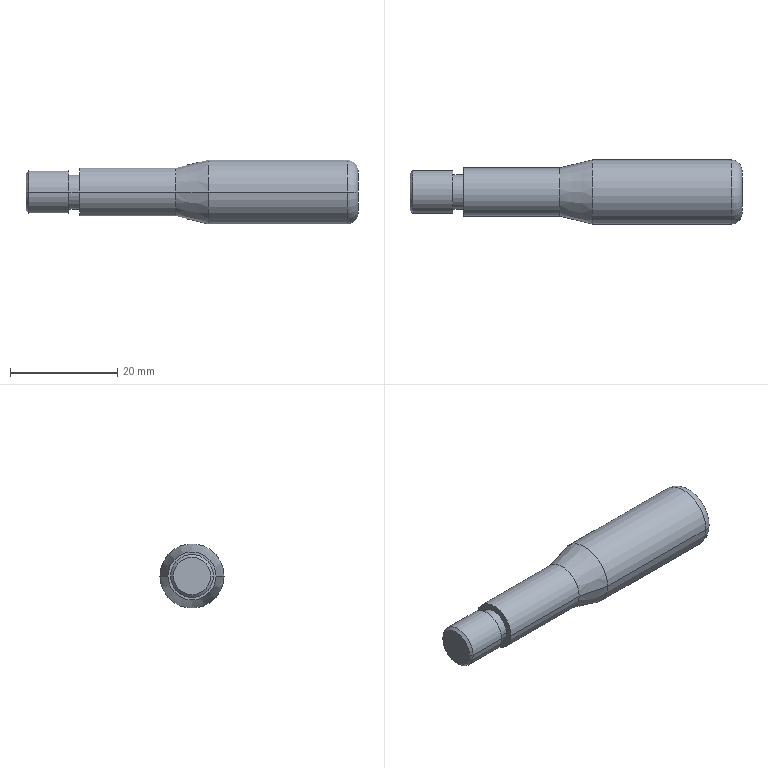Part | SolidWorks | features Chamfer 1, Fillet 1, Revolution 1 | 1 solid | 18 faces | box 62 x 12 x 12 mm | volume 5270 mm3 | cylinder 8 | cone 4 | plane 4 | torus 2 | commonest cylinder face diameters 6.5 x2 8 x2 9 x2 12 x2
STEP:
#1=CARTESIAN_POINT('',(0.,-3.5,0.));
#2=VERTEX_POINT('',#1);
#3=CARTESIAN_POINT('',(0.,3.5,0.));
#4=VERTEX_POINT('',#3);
#5=CARTESIAN_POINT('',(0.,0.,0.));
#6=DIRECTION('',(-1.,0.,0.));
#7=DIRECTION('',(0.,-1.,0.));
#8=AXIS2_PLACEMENT_3D('',#5,#6,#7);
#9=CIRCLE('',#8,3.5);
#10=EDGE_CURVE('',#2,#4,#9,.T.);
#11=ORIENTED_EDGE('',*,*,#10,.F.);
#12=CARTESIAN_POINT('',(0.5,-4.,0.));
#13=VERTEX_POINT('',#12);
#14=CARTESIAN_POINT('',(0.5,-4.,0.));
#15=DIRECTION('',(0.7071,-0.7071,0.));
#16=VECTOR('',#15,1000.);
#17=LINE('',#14,#16);
#18=EDGE_CURVE('',#2,#13,#17,.T.);
#19=ORIENTED_EDGE('',*,*,#18,.T.);
#20=CARTESIAN_POINT('',(0.5,4.,0.));
#21=VERTEX_POINT('',#20);
#22=CARTESIAN_POINT('',(0.5,0.,0.));
#23=DIRECTION('',(1.,0.,0.));
#24=DIRECTION('',(0.,-1.,0.));
#25=AXIS2_PLACEMENT_3D('',#22,#23,#24);
#26=CIRCLE('',#25,4.);
#27=EDGE_CURVE('',#21,#13,#26,.T.);
#28=ORIENTED_EDGE('',*,*,#27,.F.);
#29=CARTESIAN_POINT('',(0.5,4.,0.));
#30=DIRECTION('',(0.7071,0.7071,0.));
#31=VECTOR('',#30,1000.);
#32=LINE('',#29,#31);
#33=EDGE_CURVE('',#4,#21,#32,.T.);
#34=ORIENTED_EDGE('',*,*,#33,.F.);
#35=EDGE_LOOP('',(#11,#19,#28,#34));
#36=FACE_OUTER_BOUND('',#35,.T.);
#37=CARTESIAN_POINT('',(0.5,0.,0.));
#38=DIRECTION('',(1.,0.,0.));
#39=DIRECTION('',(0.,1.,0.));
#40=AXIS2_PLACEMENT_3D('',#37,#38,#39);
#41=CONICAL_SURFACE('',#40,4.,0.7854);
#42=ADVANCED_FACE('',(#36),#41,.T.);
#43=CARTESIAN_POINT('',(60.,-6.,0.));
#44=VERTEX_POINT('',#43);
#45=CARTESIAN_POINT('',(60.,6.,0.));
#46=VERTEX_POINT('',#45);
#47=CARTESIAN_POINT('',(60.,0.,0.));
#48=DIRECTION('',(-1.,0.,0.));
#49=DIRECTION('',(0.,1.,0.));
#50=AXIS2_PLACEMENT_3D('',#47,#48,#49);
#51=CIRCLE('',#50,6.);
#52=EDGE_CURVE('',#44,#46,#51,.T.);
#53=ORIENTED_EDGE('',*,*,#52,.F.);
#54=CARTESIAN_POINT('',(62.,-4.,0.));
#55=VERTEX_POINT('',#54);
#56=CARTESIAN_POINT('',(60.,-4.,0.));
#57=DIRECTION('',(0.,0.,1.));
#58=DIRECTION('',(0.,-1.,0.));
#59=AXIS2_PLACEMENT_3D('',#56,#57,#58);
#60=CIRCLE('',#59,2.);
#61=EDGE_CURVE('',#44,#55,#60,.T.);
#62=ORIENTED_EDGE('',*,*,#61,.T.);
#63=CARTESIAN_POINT('',(62.,4.,0.));
#64=VERTEX_POINT('',#63);
#65=CARTESIAN_POINT('',(62.,0.,0.));
#66=DIRECTION('',(1.,0.,0.));
#67=DIRECTION('',(0.,1.,0.));
#68=AXIS2_PLACEMENT_3D('',#65,#66,#67);
#69=CIRCLE('',#68,4.);
#70=EDGE_CURVE('',#64,#55,#69,.T.);
#71=ORIENTED_EDGE('',*,*,#70,.F.);
#72=CARTESIAN_POINT('',(60.,4.,0.));
#73=DIRECTION('',(0.,0.,-1.));
#74=DIRECTION('',(-1.,0.,0.));
#75=AXIS2_PLACEMENT_3D('',#72,#73,#74);
#76=CIRCLE('',#75,2.);
#77=EDGE_CURVE('',#46,#64,#76,.T.);
#78=ORIENTED_EDGE('',*,*,#77,.F.);
#79=EDGE_LOOP('',(#53,#62,#71,#78));
#80=FACE_OUTER_BOUND('',#79,.T.);
#81=CARTESIAN_POINT('',(60.,0.,0.));
#82=DIRECTION('',(1.,0.,0.));
#83=DIRECTION('',(0.,1.,0.));
#84=AXIS2_PLACEMENT_3D('',#81,#82,#83);
#85=TOROIDAL_SURFACE('',#84,4.,2.);
#86=ADVANCED_FACE('',(#80),#85,.T.);
#87=CARTESIAN_POINT('',(34.,6.,0.));
#88=VERTEX_POINT('',#87);
#89=CARTESIAN_POINT('',(34.,-6.,0.));
#90=VERTEX_POINT('',#89);
#91=CARTESIAN_POINT('',(34.,0.,0.));
#92=DIRECTION('',(1.,0.,0.));
#93=DIRECTION('',(0.,1.,0.));
#94=AXIS2_PLACEMENT_3D('',#91,#92,#93);
#95=CIRCLE('',#94,6.);
#96=EDGE_CURVE('',#88,#90,#95,.T.);
#97=ORIENTED_EDGE('',*,*,#96,.T.);
#98=CARTESIAN_POINT('',(62.,-6.,0.));
#99=DIRECTION('',(1.,0.,0.));
#100=VECTOR('',#99,1000.);
#101=LINE('',#98,#100);
#102=EDGE_CURVE('',#90,#44,#101,.T.);
#103=ORIENTED_EDGE('',*,*,#102,.T.);
#104=ORIENTED_EDGE('',*,*,#52,.T.);
#105=CARTESIAN_POINT('',(62.,6.,0.));
#106=DIRECTION('',(1.,0.,0.));
#107=VECTOR('',#106,1000.);
#108=LINE('',#105,#107);
#109=EDGE_CURVE('',#88,#46,#108,.T.);
#110=ORIENTED_EDGE('',*,*,#109,.F.);
#111=EDGE_LOOP('',(#97,#103,#104,#110));
#112=FACE_OUTER_BOUND('',#111,.T.);
#113=CARTESIAN_POINT('',(62.,0.,0.));
#114=DIRECTION('',(1.,0.,0.));
#115=DIRECTION('',(0.,1.,0.));
#116=AXIS2_PLACEMENT_3D('',#113,#114,#115);
#117=CYLINDRICAL_SURFACE('',#116,6.);
#118=ADVANCED_FACE('',(#112),#117,.T.);
#119=CARTESIAN_POINT('',(28.,4.5,0.));
#120=VERTEX_POINT('',#119);
#121=CARTESIAN_POINT('',(28.,-4.5,0.));
#122=VERTEX_POINT('',#121);
#123=CARTESIAN_POINT('',(28.,0.,0.));
#124=DIRECTION('',(1.,0.,0.));
#125=DIRECTION('',(0.,1.,0.));
#126=AXIS2_PLACEMENT_3D('',#123,#124,#125);
#127=CIRCLE('',#126,4.5);
#128=EDGE_CURVE('',#120,#122,#127,.T.);
#129=ORIENTED_EDGE('',*,*,#128,.T.);
#130=CARTESIAN_POINT('',(34.,-6.,0.));
#131=DIRECTION('',(0.9701,-0.2425,0.));
#132=VECTOR('',#131,1000.);
#133=LINE('',#130,#132);
#134=EDGE_CURVE('',#122,#90,#133,.T.);
#135=ORIENTED_EDGE('',*,*,#134,.T.);
#136=ORIENTED_EDGE('',*,*,#96,.F.);
#137=CARTESIAN_POINT('',(34.,6.,0.));
#138=DIRECTION('',(0.9701,0.2425,0.));
#139=VECTOR('',#138,1000.);
#140=LINE('',#137,#139);
#141=EDGE_CURVE('',#120,#88,#140,.T.);
#142=ORIENTED_EDGE('',*,*,#141,.F.);
#143=EDGE_LOOP('',(#129,#135,#136,#142));
#144=FACE_OUTER_BOUND('',#143,.T.);
#145=CARTESIAN_POINT('',(34.,0.,0.));
#146=DIRECTION('',(1.,0.,0.));
#147=DIRECTION('',(0.,1.,0.));
#148=AXIS2_PLACEMENT_3D('',#145,#146,#147);
#149=CONICAL_SURFACE('',#148,6.,0.245);
#150=ADVANCED_FACE('',(#144),#149,.T.);
#151=CARTESIAN_POINT('',(10.,4.5,0.));
#152=VERTEX_POINT('',#151);
#153=CARTESIAN_POINT('',(10.,-4.5,0.));
#154=VERTEX_POINT('',#153);
#155=CARTESIAN_POINT('',(10.,0.,0.));
#156=DIRECTION('',(1.,0.,0.));
#157=DIRECTION('',(0.,1.,0.));
#158=AXIS2_PLACEMENT_3D('',#155,#156,#157);
#159=CIRCLE('',#158,4.5);
#160=EDGE_CURVE('',#152,#154,#159,.T.);
#161=ORIENTED_EDGE('',*,*,#160,.T.);
#162=CARTESIAN_POINT('',(62.,-4.5,0.));
#163=DIRECTION('',(1.,0.,0.));
#164=VECTOR('',#163,1000.);
#165=LINE('',#162,#164);
#166=EDGE_CURVE('',#154,#122,#165,.T.);
#167=ORIENTED_EDGE('',*,*,#166,.T.);
#168=ORIENTED_EDGE('',*,*,#128,.F.);
#169=CARTESIAN_POINT('',(62.,4.5,0.));
#170=DIRECTION('',(1.,0.,0.));
#171=VECTOR('',#170,1000.);
#172=LINE('',#169,#171);
#173=EDGE_CURVE('',#152,#120,#172,.T.);
#174=ORIENTED_EDGE('',*,*,#173,.F.);
#175=EDGE_LOOP('',(#161,#167,#168,#174));
#176=FACE_OUTER_BOUND('',#175,.T.);
#177=CARTESIAN_POINT('',(62.,0.,0.));
#178=DIRECTION('',(1.,0.,0.));
#179=DIRECTION('',(0.,1.,0.));
#180=AXIS2_PLACEMENT_3D('',#177,#178,#179);
#181=CYLINDRICAL_SURFACE('',#180,4.5);
#182=ADVANCED_FACE('',(#176),#181,.T.);
#183=CARTESIAN_POINT('',(8.,3.25,0.));
#184=VERTEX_POINT('',#183);
#185=CARTESIAN_POINT('',(8.,-3.25,0.));
#186=VERTEX_POINT('',#185);
#187=CARTESIAN_POINT('',(8.,0.,0.));
#188=DIRECTION('',(1.,0.,0.));
#189=DIRECTION('',(0.,1.,0.));
#190=AXIS2_PLACEMENT_3D('',#187,#188,#189);
#191=CIRCLE('',#190,3.25);
#192=EDGE_CURVE('',#184,#186,#191,.T.);
#193=ORIENTED_EDGE('',*,*,#192,.T.);
#194=CARTESIAN_POINT('',(10.,-3.25,0.));
#195=VERTEX_POINT('',#194);
#196=CARTESIAN_POINT('',(62.,-3.25,0.));
#197=DIRECTION('',(1.,0.,0.));
#198=VECTOR('',#197,1000.);
#199=LINE('',#196,#198);
#200=EDGE_CURVE('',#186,#195,#199,.T.);
#201=ORIENTED_EDGE('',*,*,#200,.T.);
#202=CARTESIAN_POINT('',(10.,3.25,0.));
#203=VERTEX_POINT('',#202);
#204=CARTESIAN_POINT('',(10.,0.,0.));
#205=DIRECTION('',(1.,0.,0.));
#206=DIRECTION('',(0.,1.,0.));
#207=AXIS2_PLACEMENT_3D('',#204,#205,#206);
#208=CIRCLE('',#207,3.25);
#209=EDGE_CURVE('',#203,#195,#208,.T.);
#210=ORIENTED_EDGE('',*,*,#209,.F.);
#211=CARTESIAN_POINT('',(62.,3.25,0.));
#212=DIRECTION('',(1.,0.,0.));
#213=VECTOR('',#212,1000.);
#214=LINE('',#211,#213);
#215=EDGE_CURVE('',#184,#203,#214,.T.);
#216=ORIENTED_EDGE('',*,*,#215,.F.);
#217=EDGE_LOOP('',(#193,#201,#210,#216));
#218=FACE_OUTER_BOUND('',#217,.T.);
#219=CARTESIAN_POINT('',(62.,0.,0.));
#220=DIRECTION('',(1.,0.,0.));
#221=DIRECTION('',(0.,1.,0.));
#222=AXIS2_PLACEMENT_3D('',#219,#220,#221);
#223=CYLINDRICAL_SURFACE('',#222,3.25);
#224=ADVANCED_FACE('',(#218),#223,.T.);
#225=ORIENTED_EDGE('',*,*,#27,.T.);
#226=CARTESIAN_POINT('',(8.,-4.,0.));
#227=VERTEX_POINT('',#226);
#228=CARTESIAN_POINT('',(62.,-4.,0.));
#229=DIRECTION('',(1.,0.,0.));
#230=VECTOR('',#229,1000.);
#231=LINE('',#228,#230);
#232=EDGE_CURVE('',#13,#227,#231,.T.);
#233=ORIENTED_EDGE('',*,*,#232,.T.);
#234=CARTESIAN_POINT('',(8.,4.,0.));
#235=VERTEX_POINT('',#234);
#236=CARTESIAN_POINT('',(8.,0.,0.));
#237=DIRECTION('',(1.,0.,0.));
#238=DIRECTION('',(0.,1.,0.));
#239=AXIS2_PLACEMENT_3D('',#236,#237,#238);
#240=CIRCLE('',#239,4.);
#241=EDGE_CURVE('',#235,#227,#240,.T.);
#242=ORIENTED_EDGE('',*,*,#241,.F.);
#243=CARTESIAN_POINT('',(62.,4.,0.));
#244=DIRECTION('',(1.,0.,0.));
#245=VECTOR('',#244,1000.);
#246=LINE('',#243,#245);
#247=EDGE_CURVE('',#21,#235,#246,.T.);
#248=ORIENTED_EDGE('',*,*,#247,.F.);
#249=EDGE_LOOP('',(#225,#233,#242,#248));
#250=FACE_OUTER_BOUND('',#249,.T.);
#251=CARTESIAN_POINT('',(62.,0.,0.));
#252=DIRECTION('',(1.,0.,0.));
#253=DIRECTION('',(0.,1.,0.));
#254=AXIS2_PLACEMENT_3D('',#251,#252,#253);
#255=CYLINDRICAL_SURFACE('',#254,4.);
#256=ADVANCED_FACE('',(#250),#255,.T.);
#257=CARTESIAN_POINT('',(0.,0.,0.));
#258=DIRECTION('',(-1.,0.,0.));
#259=DIRECTION('',(0.,-1.,0.));
#260=AXIS2_PLACEMENT_3D('',#257,#258,#259);
#261=CIRCLE('',#260,3.5);
#262=EDGE_CURVE('',#4,#2,#261,.T.);
#263=ORIENTED_EDGE('',*,*,#262,.T.);
#264=ORIENTED_EDGE('',*,*,#10,.T.);
#265=EDGE_LOOP('',(#263,#264));
#266=FACE_OUTER_BOUND('',#265,.T.);
#267=CARTESIAN_POINT('',(0.,0.,0.));
#268=DIRECTION('',(-1.,0.,0.));
#269=DIRECTION('',(0.,-1.,0.));
#270=AXIS2_PLACEMENT_3D('',#267,#268,#269);
#271=PLANE('',#270);
#272=ADVANCED_FACE('',(#266),#271,.T.);
#273=ORIENTED_EDGE('',*,*,#232,.F.);
#274=CARTESIAN_POINT('',(0.5,0.,0.));
#275=DIRECTION('',(1.,0.,0.));
#276=DIRECTION('',(0.,-1.,0.));
#277=AXIS2_PLACEMENT_3D('',#274,#275,#276);
#278=CIRCLE('',#277,4.);
#279=EDGE_CURVE('',#13,#21,#278,.T.);
#280=ORIENTED_EDGE('',*,*,#279,.T.);
#281=ORIENTED_EDGE('',*,*,#247,.T.);
#282=CARTESIAN_POINT('',(8.,0.,0.));
#283=DIRECTION('',(1.,0.,0.));
#284=DIRECTION('',(0.,1.,0.));
#285=AXIS2_PLACEMENT_3D('',#282,#283,#284);
#286=CIRCLE('',#285,4.);
#287=EDGE_CURVE('',#227,#235,#286,.T.);
#288=ORIENTED_EDGE('',*,*,#287,.F.);
#289=EDGE_LOOP('',(#273,#280,#281,#288));
#290=FACE_OUTER_BOUND('',#289,.T.);
#291=CARTESIAN_POINT('',(62.,0.,0.));
#292=DIRECTION('',(1.,0.,0.));
#293=DIRECTION('',(0.,1.,0.));
#294=AXIS2_PLACEMENT_3D('',#291,#292,#293);
#295=CYLINDRICAL_SURFACE('',#294,4.);
#296=ADVANCED_FACE('',(#290),#295,.T.);
#297=ORIENTED_EDGE('',*,*,#241,.T.);
#298=ORIENTED_EDGE('',*,*,#287,.T.);
#299=EDGE_LOOP('',(#297,#298));
#300=FACE_OUTER_BOUND('',#299,.T.);
#301=ORIENTED_EDGE('',*,*,#192,.F.);
#302=CARTESIAN_POINT('',(8.,0.,0.));
#303=DIRECTION('',(1.,0.,0.));
#304=DIRECTION('',(0.,1.,0.));
#305=AXIS2_PLACEMENT_3D('',#302,#303,#304);
#306=CIRCLE('',#305,3.25);
#307=EDGE_CURVE('',#186,#184,#306,.T.);
#308=ORIENTED_EDGE('',*,*,#307,.F.);
#309=EDGE_LOOP('',(#301,#308));
#310=FACE_BOUND('',#309,.T.);
#311=CARTESIAN_POINT('',(8.,4.,0.));
#312=DIRECTION('',(1.,0.,0.));
#313=DIRECTION('',(0.,1.,0.));
#314=AXIS2_PLACEMENT_3D('',#311,#312,#313);
#315=PLANE('',#314);
#316=ADVANCED_FACE('',(#300,#310),#315,.T.);
#317=ORIENTED_EDGE('',*,*,#200,.F.);
#318=ORIENTED_EDGE('',*,*,#307,.T.);
#319=ORIENTED_EDGE('',*,*,#215,.T.);
#320=CARTESIAN_POINT('',(10.,0.,0.));
#321=DIRECTION('',(1.,0.,0.));
#322=DIRECTION('',(0.,1.,0.));
#323=AXIS2_PLACEMENT_3D('',#320,#321,#322);
#324=CIRCLE('',#323,3.25);
#325=EDGE_CURVE('',#195,#203,#324,.T.);
#326=ORIENTED_EDGE('',*,*,#325,.F.);
#327=EDGE_LOOP('',(#317,#318,#319,#326));
#328=FACE_OUTER_BOUND('',#327,.T.);
#329=CARTESIAN_POINT('',(62.,0.,0.));
#330=DIRECTION('',(1.,0.,0.));
#331=DIRECTION('',(0.,1.,0.));
#332=AXIS2_PLACEMENT_3D('',#329,#330,#331);
#333=CYLINDRICAL_SURFACE('',#332,3.25);
#334=ADVANCED_FACE('',(#328),#333,.T.);
#335=ORIENTED_EDGE('',*,*,#209,.T.);
#336=ORIENTED_EDGE('',*,*,#325,.T.);
#337=EDGE_LOOP('',(#335,#336));
#338=FACE_BOUND('',#337,.T.);
#339=ORIENTED_EDGE('',*,*,#160,.F.);
#340=CARTESIAN_POINT('',(10.,0.,0.));
#341=DIRECTION('',(1.,0.,0.));
#342=DIRECTION('',(0.,1.,0.));
#343=AXIS2_PLACEMENT_3D('',#340,#341,#342);
#344=CIRCLE('',#343,4.5);
#345=EDGE_CURVE('',#154,#152,#344,.T.);
#346=ORIENTED_EDGE('',*,*,#345,.F.);
#347=EDGE_LOOP('',(#339,#346));
#348=FACE_OUTER_BOUND('',#347,.T.);
#349=CARTESIAN_POINT('',(10.,3.25,0.));
#350=DIRECTION('',(-1.,0.,0.));
#351=DIRECTION('',(0.,-1.,0.));
#352=AXIS2_PLACEMENT_3D('',#349,#350,#351);
#353=PLANE('',#352);
#354=ADVANCED_FACE('',(#338,#348),#353,.T.);
#355=ORIENTED_EDGE('',*,*,#166,.F.);
#356=ORIENTED_EDGE('',*,*,#345,.T.);
#357=ORIENTED_EDGE('',*,*,#173,.T.);
#358=CARTESIAN_POINT('',(28.,0.,0.));
#359=DIRECTION('',(1.,0.,0.));
#360=DIRECTION('',(0.,1.,0.));
#361=AXIS2_PLACEMENT_3D('',#358,#359,#360);
#362=CIRCLE('',#361,4.5);
#363=EDGE_CURVE('',#122,#120,#362,.T.);
#364=ORIENTED_EDGE('',*,*,#363,.F.);
#365=EDGE_LOOP('',(#355,#356,#357,#364));
#366=FACE_OUTER_BOUND('',#365,.T.);
#367=CARTESIAN_POINT('',(62.,0.,0.));
#368=DIRECTION('',(1.,0.,0.));
#369=DIRECTION('',(0.,1.,0.));
#370=AXIS2_PLACEMENT_3D('',#367,#368,#369);
#371=CYLINDRICAL_SURFACE('',#370,4.5);
#372=ADVANCED_FACE('',(#366),#371,.T.);
#373=ORIENTED_EDGE('',*,*,#134,.F.);
#374=ORIENTED_EDGE('',*,*,#363,.T.);
#375=ORIENTED_EDGE('',*,*,#141,.T.);
#376=CARTESIAN_POINT('',(34.,0.,0.));
#377=DIRECTION('',(1.,0.,0.));
#378=DIRECTION('',(0.,1.,0.));
#379=AXIS2_PLACEMENT_3D('',#376,#377,#378);
#380=CIRCLE('',#379,6.);
#381=EDGE_CURVE('',#90,#88,#380,.T.);
#382=ORIENTED_EDGE('',*,*,#381,.F.);
#383=EDGE_LOOP('',(#373,#374,#375,#382));
#384=FACE_OUTER_BOUND('',#383,.T.);
#385=CARTESIAN_POINT('',(34.,0.,0.));
#386=DIRECTION('',(1.,0.,0.));
#387=DIRECTION('',(0.,1.,0.));
#388=AXIS2_PLACEMENT_3D('',#385,#386,#387);
#389=CONICAL_SURFACE('',#388,6.,0.245);
#390=ADVANCED_FACE('',(#384),#389,.T.);
#391=ORIENTED_EDGE('',*,*,#102,.F.);
#392=ORIENTED_EDGE('',*,*,#381,.T.);
#393=ORIENTED_EDGE('',*,*,#109,.T.);
#394=CARTESIAN_POINT('',(60.,0.,0.));
#395=DIRECTION('',(-1.,0.,0.));
#396=DIRECTION('',(0.,1.,0.));
#397=AXIS2_PLACEMENT_3D('',#394,#395,#396);
#398=CIRCLE('',#397,6.);
#399=EDGE_CURVE('',#46,#44,#398,.T.);
#400=ORIENTED_EDGE('',*,*,#399,.T.);
#401=EDGE_LOOP('',(#391,#392,#393,#400));
#402=FACE_OUTER_BOUND('',#401,.T.);
#403=CARTESIAN_POINT('',(62.,0.,0.));
#404=DIRECTION('',(1.,0.,0.));
#405=DIRECTION('',(0.,1.,0.));
#406=AXIS2_PLACEMENT_3D('',#403,#404,#405);
#407=CYLINDRICAL_SURFACE('',#406,6.);
#408=ADVANCED_FACE('',(#402),#407,.T.);
#409=ORIENTED_EDGE('',*,*,#70,.T.);
#410=CARTESIAN_POINT('',(62.,0.,0.));
#411=DIRECTION('',(1.,0.,0.));
#412=DIRECTION('',(0.,1.,0.));
#413=AXIS2_PLACEMENT_3D('',#410,#411,#412);
#414=CIRCLE('',#413,4.);
#415=EDGE_CURVE('',#55,#64,#414,.T.);
#416=ORIENTED_EDGE('',*,*,#415,.T.);
#417=EDGE_LOOP('',(#409,#416));
#418=FACE_OUTER_BOUND('',#417,.T.);
#419=CARTESIAN_POINT('',(62.,6.,0.));
#420=DIRECTION('',(1.,0.,0.));
#421=DIRECTION('',(0.,1.,0.));
#422=AXIS2_PLACEMENT_3D('',#419,#420,#421);
#423=PLANE('',#422);
#424=ADVANCED_FACE('',(#418),#423,.T.);
#425=ORIENTED_EDGE('',*,*,#61,.F.);
#426=ORIENTED_EDGE('',*,*,#399,.F.);
#427=ORIENTED_EDGE('',*,*,#77,.T.);
#428=ORIENTED_EDGE('',*,*,#415,.F.);
#429=EDGE_LOOP('',(#425,#426,#427,#428));
#430=FACE_OUTER_BOUND('',#429,.T.);
#431=CARTESIAN_POINT('',(60.,0.,0.));
#432=DIRECTION('',(1.,0.,0.));
#433=DIRECTION('',(0.,1.,0.));
#434=AXIS2_PLACEMENT_3D('',#431,#432,#433);
#435=TOROIDAL_SURFACE('',#434,4.,2.);
#436=ADVANCED_FACE('',(#430),#435,.T.);
#437=ORIENTED_EDGE('',*,*,#18,.F.);
#438=ORIENTED_EDGE('',*,*,#262,.F.);
#439=ORIENTED_EDGE('',*,*,#33,.T.);
#440=ORIENTED_EDGE('',*,*,#279,.F.);
#441=EDGE_LOOP('',(#437,#438,#439,#440));
#442=FACE_OUTER_BOUND('',#441,.T.);
#443=CARTESIAN_POINT('',(0.5,0.,0.));
#444=DIRECTION('',(1.,0.,0.));
#445=DIRECTION('',(0.,1.,0.));
#446=AXIS2_PLACEMENT_3D('',#443,#444,#445);
#447=CONICAL_SURFACE('',#446,4.,0.7854);
#448=ADVANCED_FACE('',(#442),#447,.T.);
#449=CLOSED_SHELL('',(#42,#86,#118,#150,#182,#224,#256,#272,#296,#316,#334,#354,#372,#390,#408,#424,#436,#448));
#450=MANIFOLD_SOLID_BREP('',#449);
#451=CARTESIAN_POINT('',(0.,0.,0.));
#452=DIRECTION('',(0.,0.,1.));
#453=DIRECTION('',(1.,0.,0.));
#454=AXIS2_PLACEMENT_3D('',#451,#452,#453);
#455=(LENGTH_UNIT()NAMED_UNIT(*)SI_UNIT(.MILLI.,.METRE.));
#456=UNCERTAINTY_MEASURE_WITH_UNIT(LENGTH_MEASURE(0.00001),#455,'','');
#457=(NAMED_UNIT(*)PLANE_ANGLE_UNIT()SI_UNIT($,.RADIAN.));
#458=(NAMED_UNIT(*)SI_UNIT($,.STERADIAN.)SOLID_ANGLE_UNIT());
#459=(GEOMETRIC_REPRESENTATION_CONTEXT(3)GLOBAL_UNCERTAINTY_ASSIGNED_CONTEXT((#456))GLOBAL_UNIT_ASSIGNED_CONTEXT((#455,#457,#458))REPRESENTATION_CONTEXT('',''));
#460=ADVANCED_BREP_SHAPE_REPRESENTATION('',(#450,#454),#459);